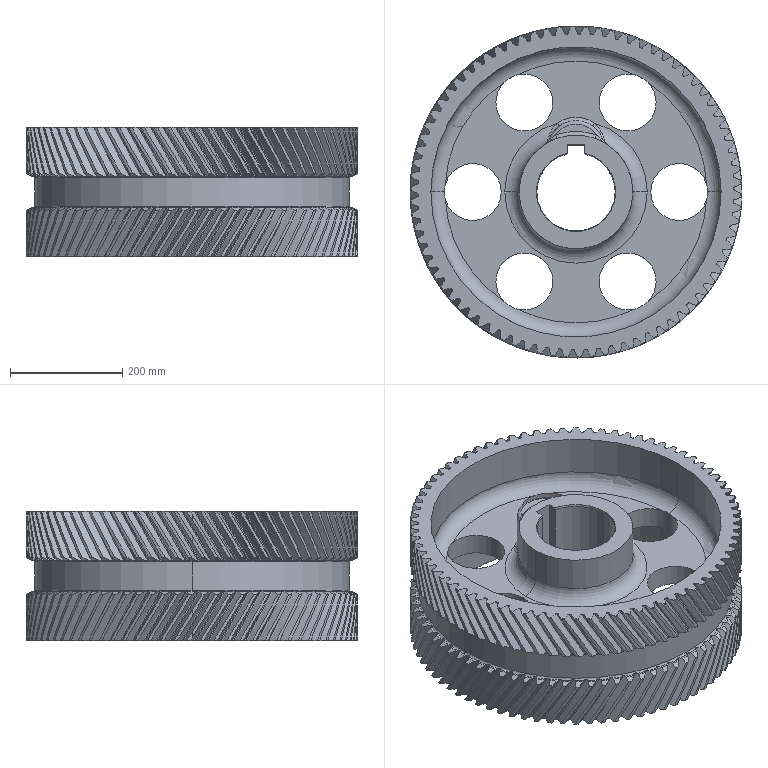Part | SolidWorks | features ICE 4, Chamfer 3, Fillet 3, CirPattern 1, Extrusion 1, Helix 1, MirrorSolid 1, RefAxis 1, RevCut 1, SweepCut 1 | 1 solid | 1188 faces | box 591.617 x 591.617 x 230.532 mm | volume 20474904 mm3 | spline 484 | cone 320 | cylinder 193 | plane 167 | torus 24 | commonest cylinder face diameters 591.617 x160 101.6 x14 203.2 x6 50.8 x4 517.65 x4 139.624 x3